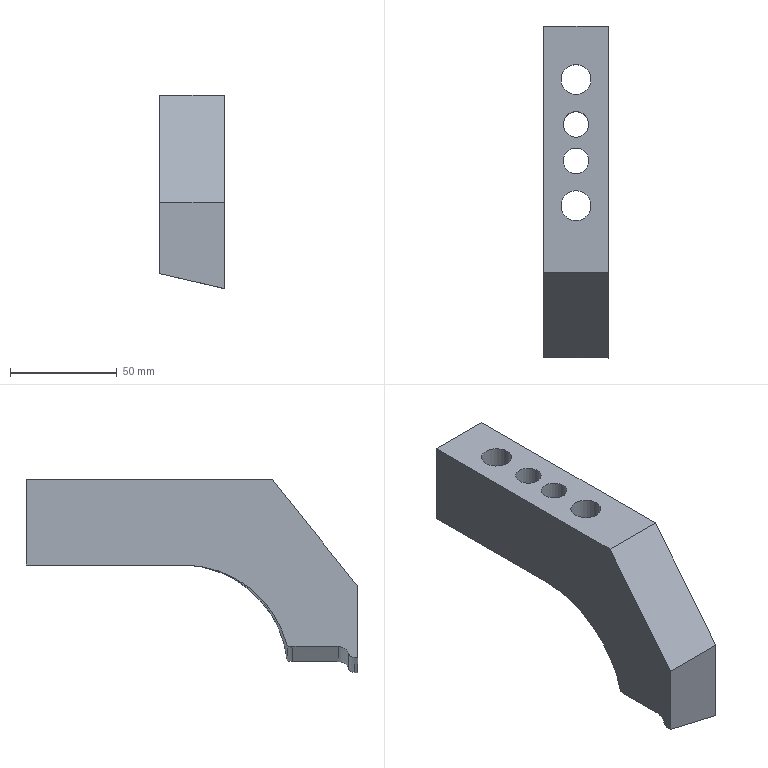Part | NX | features solid 2 | 1 solid | 21 faces | box 30 x 155 x 90.276 mm | volume 186324 mm3 | plane 8 | spline 7 | cylinder 6 | commonest cylinder face diameters 12 x2 14 x2 20 x2
STEP:
#1=CARTESIAN_POINT('',(-556.,-381.,60.));
#2=VERTEX_POINT('',#1);
#3=CARTESIAN_POINT('',(-550.,-381.,60.));
#4=DIRECTION('',(0.,0.,-1.));
#5=DIRECTION('',(-1.,0.,0.));
#6=AXIS2_PLACEMENT_3D('',#3,#4,#5);
#7=CIRCLE('',#6,6.);
#8=EDGE_CURVE('',#2,#2,#7,.T.);
#9=ORIENTED_EDGE('',*,*,#8,.F.);
#10=EDGE_LOOP('',(#9));
#11=FACE_BOUND('',#10,.T.);
#12=CARTESIAN_POINT('',(-556.,-364.,60.));
#13=VERTEX_POINT('',#12);
#14=CARTESIAN_POINT('',(-550.,-364.,60.));
#15=DIRECTION('',(0.,0.,-1.));
#16=DIRECTION('',(-1.,0.,0.));
#17=AXIS2_PLACEMENT_3D('',#14,#15,#16);
#18=CIRCLE('',#17,6.);
#19=EDGE_CURVE('',#13,#13,#18,.T.);
#20=ORIENTED_EDGE('',*,*,#19,.F.);
#21=EDGE_LOOP('',(#20));
#22=FACE_BOUND('',#21,.T.);
#23=CARTESIAN_POINT('',(-560.,-343.,60.));
#24=VERTEX_POINT('',#23);
#25=CARTESIAN_POINT('',(-550.,-343.,60.));
#26=DIRECTION('',(0.,0.,-1.));
#27=DIRECTION('',(-1.,0.,0.));
#28=AXIS2_PLACEMENT_3D('',#25,#26,#27);
#29=CIRCLE('',#28,10.);
#30=EDGE_CURVE('',#24,#24,#29,.F.);
#31=ORIENTED_EDGE('',*,*,#30,.T.);
#32=EDGE_LOOP('',(#31));
#33=FACE_BOUND('',#32,.T.);
#34=CARTESIAN_POINT('',(-535.,-390.262,60.));
#35=VERTEX_POINT('',#34);
#36=CARTESIAN_POINT('',(-535.,-318.,60.));
#37=VERTEX_POINT('',#36);
#38=CARTESIAN_POINT('',(-535.,-449.758,60.));
#39=DIRECTION('',(0.,1.,0.));
#40=VECTOR('',#39,1000.);
#41=LINE('',#38,#40);
#42=EDGE_CURVE('',#35,#37,#41,.T.);
#43=ORIENTED_EDGE('',*,*,#42,.F.);
#44=CARTESIAN_POINT('',(-565.,-391.431,60.));
#45=VERTEX_POINT('',#44);
#46=CARTESIAN_POINT('',(-535.,-390.262,60.));
#47=CARTESIAN_POINT('',(-545.006,-390.49,60.));
#48=CARTESIAN_POINT('',(-555.007,-390.87,60.));
#49=CARTESIAN_POINT('',(-565.,-391.431,60.));
#50=B_SPLINE_CURVE_WITH_KNOTS('',3,(#46,#47,#48,#49),.UNSPECIFIED.,.F.,.F.,(4,4),(0.,0.03002),.UNSPECIFIED.);
#51=EDGE_CURVE('',#35,#45,#50,.T.);
#52=ORIENTED_EDGE('',*,*,#51,.T.);
#53=CARTESIAN_POINT('',(-565.,-318.,60.));
#54=VERTEX_POINT('',#53);
#55=CARTESIAN_POINT('',(-565.,-425.,60.));
#56=DIRECTION('',(0.,1.,0.));
#57=VECTOR('',#56,1000.);
#58=LINE('',#55,#57);
#59=EDGE_CURVE('',#45,#54,#58,.T.);
#60=ORIENTED_EDGE('',*,*,#59,.T.);
#61=CARTESIAN_POINT('',(-535.,-318.,60.));
#62=CARTESIAN_POINT('',(-545.,-318.,60.));
#63=CARTESIAN_POINT('',(-555.,-318.,60.));
#64=CARTESIAN_POINT('',(-565.,-318.,60.));
#65=B_SPLINE_CURVE_WITH_KNOTS('',3,(#61,#62,#63,#64),.UNSPECIFIED.,.F.,.F.,(4,4),(0.,0.03),.UNSPECIFIED.);
#66=EDGE_CURVE('',#37,#54,#65,.T.);
#67=ORIENTED_EDGE('',*,*,#66,.F.);
#68=EDGE_LOOP('',(#43,#52,#60,#67));
#69=FACE_BOUND('',#68,.T.);
#70=CARTESIAN_POINT('',(-535.,-425.,60.));
#71=DIRECTION('',(0.,0.,-1.));
#72=DIRECTION('',(-1.,0.,0.));
#73=AXIS2_PLACEMENT_3D('',#70,#71,#72);
#74=PLANE('',#73);
#75=ADVANCED_FACE('',(#11,#22,#33,#69),#74,.T.);
#76=CARTESIAN_POINT('',(-565.,-473.,16.731));
#77=VERTEX_POINT('',#76);
#78=CARTESIAN_POINT('',(-565.,-473.,50.));
#79=VERTEX_POINT('',#78);
#80=CARTESIAN_POINT('',(-565.,-473.,75.));
#81=DIRECTION('',(0.,0.,-1.));
#82=VECTOR('',#81,1000.);
#83=LINE('',#80,#82);
#84=EDGE_CURVE('',#77,#79,#83,.F.);
#85=ORIENTED_EDGE('',*,*,#84,.T.);
#86=CARTESIAN_POINT('',(-565.,-433.,100.));
#87=VERTEX_POINT('',#86);
#88=CARTESIAN_POINT('',(-565.,-473.,50.));
#89=DIRECTION('',(0.,0.6247,0.7809));
#90=VECTOR('',#89,1000.);
#91=LINE('',#88,#90);
#92=EDGE_CURVE('',#79,#87,#91,.T.);
#93=ORIENTED_EDGE('',*,*,#92,.T.);
#94=CARTESIAN_POINT('',(-565.,-318.,100.));
#95=VERTEX_POINT('',#94);
#96=CARTESIAN_POINT('',(-565.,-425.,100.));
#97=DIRECTION('',(0.,-1.,0.));
#98=VECTOR('',#97,1000.);
#99=LINE('',#96,#98);
#100=EDGE_CURVE('',#87,#95,#99,.F.);
#101=ORIENTED_EDGE('',*,*,#100,.T.);
#102=CARTESIAN_POINT('',(-565.,-318.,60.));
#103=CARTESIAN_POINT('',(-565.,-318.,73.333));
#104=CARTESIAN_POINT('',(-565.,-318.,86.667));
#105=CARTESIAN_POINT('',(-565.,-318.,100.));
#106=B_SPLINE_CURVE_WITH_KNOTS('',3,(#102,#103,#104,#105),.UNSPECIFIED.,.F.,.F.,(4,4),(0.,0.04),.UNSPECIFIED.);
#107=EDGE_CURVE('',#54,#95,#106,.T.);
#108=ORIENTED_EDGE('',*,*,#107,.F.);
#109=ORIENTED_EDGE('',*,*,#59,.F.);
#110=CARTESIAN_POINT('',(-565.,-440.,22.203));
#111=VERTEX_POINT('',#110);
#112=CARTESIAN_POINT('',(-565.,-391.431,60.));
#113=CARTESIAN_POINT('',(-565.,-394.218,60.));
#114=CARTESIAN_POINT('',(-565.,-399.704,59.542));
#115=CARTESIAN_POINT('',(-565.,-407.765,57.509));
#116=CARTESIAN_POINT('',(-565.,-415.388,54.167));
#117=CARTESIAN_POINT('',(-565.,-422.329,49.641));
#118=CARTESIAN_POINT('',(-565.,-428.468,43.994));
#119=CARTESIAN_POINT('',(-565.,-433.553,37.471));
#120=CARTESIAN_POINT('',(-565.,-437.533,30.115));
#121=CARTESIAN_POINT('',(-565.,-439.319,24.906));
#122=CARTESIAN_POINT('',(-565.,-440.,22.203));
#123=B_SPLINE_CURVE_WITH_KNOTS('',3,(#112,#113,#114,#115,#116,#117,#118,#119,#120,#121,#122),.UNSPECIFIED.,.F.,.F.,(4,1,1,1,1,1,1,1,4),(0.,0.008243,0.01649,0.02473,0.03297,0.04121,0.04946,0.0577,0.06594),.UNSPECIFIED.);
#124=EDGE_CURVE('',#45,#111,#123,.T.);
#125=ORIENTED_EDGE('',*,*,#124,.T.);
#126=CARTESIAN_POINT('',(-565.,-442.207,21.944));
#127=VERTEX_POINT('',#126);
#128=CARTESIAN_POINT('',(-565.,-442.207,21.944));
#129=CARTESIAN_POINT('',(-565.,-441.46,21.946));
#130=CARTESIAN_POINT('',(-565.,-440.725,22.033));
#131=CARTESIAN_POINT('',(-565.,-440.,22.203));
#132=B_SPLINE_CURVE_WITH_KNOTS('',3,(#128,#129,#130,#131),.UNSPECIFIED.,.F.,.F.,(4,4),(0.000000091,0.002222),.UNSPECIFIED.);
#133=EDGE_CURVE('',#127,#111,#132,.T.);
#134=ORIENTED_EDGE('',*,*,#133,.F.);
#135=CARTESIAN_POINT('',(-565.,-464.022,21.891));
#136=VERTEX_POINT('',#135);
#137=CARTESIAN_POINT('',(-565.,-442.207,21.944));
#138=CARTESIAN_POINT('',(-565.,-449.479,21.926));
#139=CARTESIAN_POINT('',(-565.,-456.751,21.909));
#140=CARTESIAN_POINT('',(-565.,-464.022,21.891));
#141=B_SPLINE_CURVE_WITH_KNOTS('',3,(#137,#138,#139,#140),.UNSPECIFIED.,.F.,.F.,(4,4),(0.01263,0.03445),.UNSPECIFIED.);
#142=EDGE_CURVE('',#127,#136,#141,.T.);
#143=ORIENTED_EDGE('',*,*,#142,.T.);
#144=CARTESIAN_POINT('',(-565.,-468.65,18.668));
#145=VERTEX_POINT('',#144);
#146=CARTESIAN_POINT('',(-565.,-464.022,21.891));
#147=CARTESIAN_POINT('',(-565.,-466.037,21.887));
#148=CARTESIAN_POINT('',(-565.,-467.918,20.542));
#149=CARTESIAN_POINT('',(-565.,-468.65,18.668));
#150=B_SPLINE_CURVE_WITH_KNOTS('',3,(#146,#147,#148,#149),.UNSPECIFIED.,.F.,.F.,(4,4),(0.,0.005956),.UNSPECIFIED.);
#151=EDGE_CURVE('',#136,#145,#150,.T.);
#152=ORIENTED_EDGE('',*,*,#151,.T.);
#153=CARTESIAN_POINT('',(-565.,-471.431,16.734));
#154=VERTEX_POINT('',#153);
#155=CARTESIAN_POINT('',(-565.,-471.428,16.734));
#156=CARTESIAN_POINT('',(-565.,-470.829,16.737));
#157=CARTESIAN_POINT('',(-565.,-469.576,17.031));
#158=CARTESIAN_POINT('',(-565.,-468.869,18.107));
#159=CARTESIAN_POINT('',(-565.,-468.651,18.667));
#160=B_SPLINE_CURVE_WITH_KNOTS('',3,(#155,#156,#157,#158,#159),.UNSPECIFIED.,.F.,.F.,(4,1,4),(0.001586,0.003375,0.005164),.UNSPECIFIED.);
#161=EDGE_CURVE('',#154,#145,#160,.T.);
#162=ORIENTED_EDGE('',*,*,#161,.F.);
#163=CARTESIAN_POINT('',(-565.,-471.437,16.734));
#164=CARTESIAN_POINT('',(-565.,-471.958,16.733));
#165=CARTESIAN_POINT('',(-565.,-472.479,16.732));
#166=CARTESIAN_POINT('',(-565.,-473.,16.731));
#167=B_SPLINE_CURVE_WITH_KNOTS('',3,(#163,#164,#165,#166),.UNSPECIFIED.,.F.,.F.,(4,4),(0.005792,0.007355),.UNSPECIFIED.);
#168=EDGE_CURVE('',#154,#77,#167,.T.);
#169=ORIENTED_EDGE('',*,*,#168,.T.);
#170=EDGE_LOOP('',(#85,#93,#101,#108,#109,#125,#134,#143,#152,#162,#169));
#171=FACE_BOUND('',#170,.T.);
#172=CARTESIAN_POINT('',(-565.,-425.,75.));
#173=DIRECTION('',(1.,0.,0.));
#174=DIRECTION('',(0.,0.,-1.));
#175=AXIS2_PLACEMENT_3D('',#172,#173,#174);
#176=PLANE('',#175);
#177=ADVANCED_FACE('',(#171),#176,.F.);
#178=CARTESIAN_POINT('',(-535.,-433.,100.));
#179=VERTEX_POINT('',#178);
#180=CARTESIAN_POINT('',(-535.,-318.,100.));
#181=VERTEX_POINT('',#180);
#182=CARTESIAN_POINT('',(-535.,-425.,100.));
#183=DIRECTION('',(0.,-1.,0.));
#184=VECTOR('',#183,1000.);
#185=LINE('',#182,#184);
#186=EDGE_CURVE('',#179,#181,#185,.F.);
#187=ORIENTED_EDGE('',*,*,#186,.F.);
#188=CARTESIAN_POINT('',(-535.,-473.,50.));
#189=VERTEX_POINT('',#188);
#190=CARTESIAN_POINT('',(-535.,-585.881,-91.102));
#191=DIRECTION('',(0.,-0.6247,-0.7809));
#192=VECTOR('',#191,1000.);
#193=LINE('',#190,#192);
#194=EDGE_CURVE('',#179,#189,#193,.T.);
#195=ORIENTED_EDGE('',*,*,#194,.T.);
#196=CARTESIAN_POINT('',(-535.,-473.,9.724));
#197=VERTEX_POINT('',#196);
#198=CARTESIAN_POINT('',(-535.,-473.,-200.));
#199=DIRECTION('',(0.,0.,-1.));
#200=VECTOR('',#199,1000.);
#201=LINE('',#198,#200);
#202=EDGE_CURVE('',#197,#189,#201,.F.);
#203=ORIENTED_EDGE('',*,*,#202,.F.);
#204=CARTESIAN_POINT('',(-535.,-471.431,9.728));
#205=VERTEX_POINT('',#204);
#206=CARTESIAN_POINT('',(-535.,-471.438,9.728));
#207=CARTESIAN_POINT('',(-535.,-471.959,9.726));
#208=CARTESIAN_POINT('',(-535.,-472.479,9.725));
#209=CARTESIAN_POINT('',(-535.,-473.,9.724));
#210=B_SPLINE_CURVE_WITH_KNOTS('',3,(#206,#207,#208,#209),.UNSPECIFIED.,.F.,.F.,(4,4),(0.005813,0.007375),.UNSPECIFIED.);
#211=EDGE_CURVE('',#205,#197,#210,.T.);
#212=ORIENTED_EDGE('',*,*,#211,.F.);
#213=CARTESIAN_POINT('',(-535.,-468.651,11.657));
#214=VERTEX_POINT('',#213);
#215=CARTESIAN_POINT('',(-535.,-471.428,9.728));
#216=CARTESIAN_POINT('',(-535.,-470.823,9.731));
#217=CARTESIAN_POINT('',(-535.,-469.58,10.023));
#218=CARTESIAN_POINT('',(-535.,-468.869,11.097));
#219=CARTESIAN_POINT('',(-535.,-468.651,11.656));
#220=B_SPLINE_CURVE_WITH_KNOTS('',3,(#215,#216,#217,#218,#219),.UNSPECIFIED.,.F.,.F.,(4,1,4),(0.001587,0.003388,0.005189),.UNSPECIFIED.);
#221=EDGE_CURVE('',#205,#214,#220,.T.);
#222=ORIENTED_EDGE('',*,*,#221,.T.);
#223=CARTESIAN_POINT('',(-535.,-464.022,14.875));
#224=VERTEX_POINT('',#223);
#225=CARTESIAN_POINT('',(-535.,-464.022,14.875));
#226=CARTESIAN_POINT('',(-535.,-466.035,14.87));
#227=CARTESIAN_POINT('',(-535.,-467.917,13.53));
#228=CARTESIAN_POINT('',(-535.,-468.65,11.658));
#229=B_SPLINE_CURVE_WITH_KNOTS('',3,(#225,#226,#227,#228),.UNSPECIFIED.,.F.,.F.,(4,4),(0.,0.005952),.UNSPECIFIED.);
#230=EDGE_CURVE('',#224,#214,#229,.T.);
#231=ORIENTED_EDGE('',*,*,#230,.F.);
#232=CARTESIAN_POINT('',(-535.,-442.454,14.927));
#233=VERTEX_POINT('',#232);
#234=CARTESIAN_POINT('',(-535.,-442.454,14.927));
#235=CARTESIAN_POINT('',(-535.,-449.644,14.909));
#236=CARTESIAN_POINT('',(-535.,-456.833,14.891));
#237=CARTESIAN_POINT('',(-535.,-464.022,14.875));
#238=B_SPLINE_CURVE_WITH_KNOTS('',3,(#234,#235,#236,#237),.UNSPECIFIED.,.F.,.F.,(4,4),(0.0129,0.03447),.UNSPECIFIED.);
#239=EDGE_CURVE('',#233,#224,#238,.T.);
#240=ORIENTED_EDGE('',*,*,#239,.F.);
#241=CARTESIAN_POINT('',(-535.,-440.,15.246));
#242=VERTEX_POINT('',#241);
#243=CARTESIAN_POINT('',(-535.,-442.454,14.927));
#244=CARTESIAN_POINT('',(-535.,-441.622,14.929));
#245=CARTESIAN_POINT('',(-535.,-440.804,15.036));
#246=CARTESIAN_POINT('',(-535.,-440.,15.246));
#247=B_SPLINE_CURVE_WITH_KNOTS('',3,(#243,#244,#245,#246),.UNSPECIFIED.,.F.,.F.,(4,4),(0.,0.002475),.UNSPECIFIED.);
#248=EDGE_CURVE('',#233,#242,#247,.T.);
#249=ORIENTED_EDGE('',*,*,#248,.T.);
#250=CARTESIAN_POINT('',(-535.,-440.,15.246));
#251=CARTESIAN_POINT('',(-535.,-439.677,18.311));
#252=CARTESIAN_POINT('',(-535.,-438.488,24.267));
#253=CARTESIAN_POINT('',(-535.,-435.058,32.858));
#254=CARTESIAN_POINT('',(-535.,-430.185,40.582));
#255=CARTESIAN_POINT('',(-535.,-423.893,47.384));
#256=CARTESIAN_POINT('',(-535.,-416.594,52.839));
#257=CARTESIAN_POINT('',(-535.,-408.272,56.946));
#258=CARTESIAN_POINT('',(-535.,-399.512,59.42));
#259=CARTESIAN_POINT('',(-535.,-393.344,60.));
#260=CARTESIAN_POINT('',(-535.,-390.262,60.));
#261=B_SPLINE_CURVE_WITH_KNOTS('',3,(#250,#251,#252,#253,#254,#255,#256,#257,#258,#259,#260),.UNSPECIFIED.,.F.,.F.,(4,1,1,1,1,1,1,1,4),(0.,0.009112,0.01822,0.02734,0.03645,0.04556,0.05467,0.06379,0.0729),.UNSPECIFIED.);
#262=EDGE_CURVE('',#242,#35,#261,.T.);
#263=ORIENTED_EDGE('',*,*,#262,.T.);
#264=ORIENTED_EDGE('',*,*,#42,.T.);
#265=CARTESIAN_POINT('',(-535.,-318.,60.));
#266=CARTESIAN_POINT('',(-535.,-318.,73.333));
#267=CARTESIAN_POINT('',(-535.,-318.,86.667));
#268=CARTESIAN_POINT('',(-535.,-318.,100.));
#269=B_SPLINE_CURVE_WITH_KNOTS('',3,(#265,#266,#267,#268),.UNSPECIFIED.,.F.,.F.,(4,4),(0.,0.04),.UNSPECIFIED.);
#270=EDGE_CURVE('',#37,#181,#269,.T.);
#271=ORIENTED_EDGE('',*,*,#270,.T.);
#272=EDGE_LOOP('',(#187,#195,#203,#212,#222,#231,#240,#249,#263,#264,#271));
#273=FACE_BOUND('',#272,.T.);
#274=CARTESIAN_POINT('',(-535.,-449.758,-200.));
#275=DIRECTION('',(1.,0.,0.));
#276=DIRECTION('',(0.,0.,-1.));
#277=AXIS2_PLACEMENT_3D('',#274,#275,#276);
#278=PLANE('',#277);
#279=ADVANCED_FACE('',(#273),#278,.T.);
#280=ORIENTED_EDGE('',*,*,#202,.T.);
#281=CARTESIAN_POINT('',(-565.,-473.,50.));
#282=DIRECTION('',(1.,0.,0.));
#283=VECTOR('',#282,1000.);
#284=LINE('',#281,#283);
#285=EDGE_CURVE('',#189,#79,#284,.F.);
#286=ORIENTED_EDGE('',*,*,#285,.T.);
#287=ORIENTED_EDGE('',*,*,#84,.F.);
#288=CARTESIAN_POINT('',(-565.,-473.,16.731));
#289=CARTESIAN_POINT('',(-555.01,-473.,14.353));
#290=CARTESIAN_POINT('',(-545.01,-473.,12.017));
#291=CARTESIAN_POINT('',(-535.,-473.,9.724));
#292=B_SPLINE_CURVE_WITH_KNOTS('',3,(#288,#289,#290,#291),.UNSPECIFIED.,.F.,.F.,(4,4),(0.,0.03081),.UNSPECIFIED.);
#293=EDGE_CURVE('',#77,#197,#292,.T.);
#294=ORIENTED_EDGE('',*,*,#293,.T.);
#295=EDGE_LOOP('',(#280,#286,#287,#294));
#296=FACE_BOUND('',#295,.T.);
#297=CARTESIAN_POINT('',(-535.,-473.,60.));
#298=DIRECTION('',(0.,-1.,0.));
#299=DIRECTION('',(-1.,0.,0.));
#300=AXIS2_PLACEMENT_3D('',#297,#298,#299);
#301=PLANE('',#300);
#302=ADVANCED_FACE('',(#296),#301,.T.);
#303=ORIENTED_EDGE('',*,*,#270,.F.);
#304=ORIENTED_EDGE('',*,*,#66,.T.);
#305=ORIENTED_EDGE('',*,*,#107,.T.);
#306=CARTESIAN_POINT('',(-535.,-318.,100.));
#307=CARTESIAN_POINT('',(-545.,-318.,100.));
#308=CARTESIAN_POINT('',(-555.,-318.,100.));
#309=CARTESIAN_POINT('',(-565.,-318.,100.));
#310=B_SPLINE_CURVE_WITH_KNOTS('',3,(#306,#307,#308,#309),.UNSPECIFIED.,.F.,.F.,(4,4),(0.,0.03),.UNSPECIFIED.);
#311=EDGE_CURVE('',#181,#95,#310,.T.);
#312=ORIENTED_EDGE('',*,*,#311,.F.);
#313=EDGE_LOOP('',(#303,#304,#305,#312));
#314=FACE_BOUND('',#313,.T.);
#315=CARTESIAN_POINT('',(-565.,-318.,100.));
#316=CARTESIAN_POINT('',(-535.,-318.,100.));
#317=CARTESIAN_POINT('',(-565.,-318.,60.));
#318=CARTESIAN_POINT('',(-535.,-318.,60.));
#319=B_SPLINE_SURFACE_WITH_KNOTS('',1,1,((#315,#316),(#317,#318)),.PLANE_SURF.,.F.,.F.,.F.,(2,2),(2,2),(0.3333,0.4137),(-3.556,-3.222),.PIECEWISE_BEZIER_KNOTS.);
#320=ADVANCED_FACE('',(#314),#319,.F.);
#321=CARTESIAN_POINT('',(-540.,-343.,75.));
#322=VERTEX_POINT('',#321);
#323=CARTESIAN_POINT('',(-550.,-343.,75.));
#324=DIRECTION('',(0.,0.,-1.));
#325=DIRECTION('',(1.,0.,0.));
#326=AXIS2_PLACEMENT_3D('',#323,#324,#325);
#327=CIRCLE('',#326,10.);
#328=EDGE_CURVE('',#322,#322,#327,.T.);
#329=ORIENTED_EDGE('',*,*,#328,.F.);
#330=EDGE_LOOP('',(#329));
#331=FACE_BOUND('',#330,.T.);
#332=ORIENTED_EDGE('',*,*,#30,.F.);
#333=EDGE_LOOP('',(#332));
#334=FACE_BOUND('',#333,.T.);
#335=CARTESIAN_POINT('',(-550.,-343.,75.));
#336=DIRECTION('',(0.,0.,-1.));
#337=DIRECTION('',(1.,0.,0.));
#338=AXIS2_PLACEMENT_3D('',#335,#336,#337);
#339=CYLINDRICAL_SURFACE('',#338,10.);
#340=ADVANCED_FACE('',(#331,#334),#339,.F.);
#341=CARTESIAN_POINT('',(-540.,-402.,75.));
#342=VERTEX_POINT('',#341);
#343=CARTESIAN_POINT('',(-550.,-402.,75.));
#344=DIRECTION('',(0.,0.,-1.));
#345=DIRECTION('',(1.,0.,0.));
#346=AXIS2_PLACEMENT_3D('',#343,#344,#345);
#347=CIRCLE('',#346,10.);
#348=EDGE_CURVE('',#342,#342,#347,.T.);
#349=ORIENTED_EDGE('',*,*,#348,.F.);
#350=EDGE_LOOP('',(#349));
#351=FACE_BOUND('',#350,.T.);
#352=CARTESIAN_POINT('',(-540.005,-401.699,58.705));
#353=VERTEX_POINT('',#352);
#354=CARTESIAN_POINT('',(-541.365,-408.115,56.844));
#355=CARTESIAN_POINT('',(-539.449,-403.012,58.517));
#356=CARTESIAN_POINT('',(-540.637,-397.798,59.499));
#357=CARTESIAN_POINT('',(-543.77,-393.388,59.985));
#358=CARTESIAN_POINT('',(-550.513,-390.886,59.985));
#359=CARTESIAN_POINT('',(-557.01,-394.007,59.981));
#360=CARTESIAN_POINT('',(-559.716,-398.695,59.478));
#361=CARTESIAN_POINT('',(-560.409,-403.985,58.477));
#362=CARTESIAN_POINT('',(-558.038,-408.878,56.801));
#363=CARTESIAN_POINT('',(-553.557,-411.624,55.503));
#364=CARTESIAN_POINT('',(-549.536,-412.263,55.118));
#365=CARTESIAN_POINT('',(-545.585,-411.262,55.527));
#366=CARTESIAN_POINT('',(-541.365,-408.115,56.844));
#367=CARTESIAN_POINT('',(-539.449,-403.012,58.517));
#368=CARTESIAN_POINT('',(-540.637,-397.798,59.499));
#369=B_SPLINE_CURVE_WITH_KNOTS('',3,(#354,#355,#356,#357,#358,#359,#360,#361,#362,#363,#364,#365,#366,#367,#368),.UNSPECIFIED.,.T.,.F.,(1,1,1,1,1,1,1,1,1,1,1,1,1,1,1,1,1,1,1),(-0.01589,-0.01192,-0.007945,0.,0.003973,0.007945,0.01589,0.02384,0.02781,0.03178,0.03973,0.0437,0.04767,0.05165,0.05562,0.06356,0.06754,0.07151,0.07945),.UNSPECIFIED.);
#370=EDGE_CURVE('',#353,#353,#369,.T.);
#371=ORIENTED_EDGE('',*,*,#370,.F.);
#372=EDGE_LOOP('',(#371));
#373=FACE_BOUND('',#372,.T.);
#374=CARTESIAN_POINT('',(-550.,-402.,75.));
#375=DIRECTION('',(0.,0.,-1.));
#376=DIRECTION('',(1.,0.,0.));
#377=AXIS2_PLACEMENT_3D('',#374,#375,#376);
#378=CYLINDRICAL_SURFACE('',#377,10.);
#379=ADVANCED_FACE('',(#351,#373),#378,.F.);
#380=ORIENTED_EDGE('',*,*,#100,.F.);
#381=CARTESIAN_POINT('',(-535.,-433.,100.));
#382=DIRECTION('',(-1.,0.,0.));
#383=VECTOR('',#382,1000.);
#384=LINE('',#381,#383);
#385=EDGE_CURVE('',#87,#179,#384,.F.);
#386=ORIENTED_EDGE('',*,*,#385,.T.);
#387=ORIENTED_EDGE('',*,*,#186,.T.);
#388=ORIENTED_EDGE('',*,*,#311,.T.);
#389=EDGE_LOOP('',(#380,#386,#387,#388));
#390=FACE_BOUND('',#389,.T.);
#391=CARTESIAN_POINT('',(-556.,-381.,100.));
#392=VERTEX_POINT('',#391);
#393=CARTESIAN_POINT('',(-550.,-381.,100.));
#394=DIRECTION('',(0.,0.,-1.));
#395=DIRECTION('',(-1.,0.,0.));
#396=AXIS2_PLACEMENT_3D('',#393,#394,#395);
#397=CIRCLE('',#396,6.);
#398=EDGE_CURVE('',#392,#392,#397,.T.);
#399=ORIENTED_EDGE('',*,*,#398,.T.);
#400=EDGE_LOOP('',(#399));
#401=FACE_BOUND('',#400,.T.);
#402=CARTESIAN_POINT('',(-556.,-364.,100.));
#403=VERTEX_POINT('',#402);
#404=CARTESIAN_POINT('',(-550.,-364.,100.));
#405=DIRECTION('',(0.,0.,-1.));
#406=DIRECTION('',(-1.,0.,0.));
#407=AXIS2_PLACEMENT_3D('',#404,#405,#406);
#408=CIRCLE('',#407,6.);
#409=EDGE_CURVE('',#403,#403,#408,.T.);
#410=ORIENTED_EDGE('',*,*,#409,.T.);
#411=EDGE_LOOP('',(#410));
#412=FACE_BOUND('',#411,.T.);
#413=CARTESIAN_POINT('',(-557.,-402.,100.));
#414=VERTEX_POINT('',#413);
#415=CARTESIAN_POINT('',(-550.,-402.,100.));
#416=DIRECTION('',(0.,0.,-1.));
#417=DIRECTION('',(-1.,0.,0.));
#418=AXIS2_PLACEMENT_3D('',#415,#416,#417);
#419=CIRCLE('',#418,7.);
#420=EDGE_CURVE('',#414,#414,#419,.T.);
#421=ORIENTED_EDGE('',*,*,#420,.T.);
#422=EDGE_LOOP('',(#421));
#423=FACE_BOUND('',#422,.T.);
#424=CARTESIAN_POINT('',(-557.,-343.,100.));
#425=VERTEX_POINT('',#424);
#426=CARTESIAN_POINT('',(-550.,-343.,100.));
#427=DIRECTION('',(0.,0.,-1.));
#428=DIRECTION('',(-1.,0.,0.));
#429=AXIS2_PLACEMENT_3D('',#426,#427,#428);
#430=CIRCLE('',#429,7.);
#431=EDGE_CURVE('',#425,#425,#430,.T.);
#432=ORIENTED_EDGE('',*,*,#431,.T.);
#433=EDGE_LOOP('',(#432));
#434=FACE_BOUND('',#433,.T.);
#435=CARTESIAN_POINT('',(-605.,-425.,100.));
#436=DIRECTION('',(0.,0.,-1.));
#437=DIRECTION('',(-1.,0.,0.));
#438=AXIS2_PLACEMENT_3D('',#435,#436,#437);
#439=PLANE('',#438);
#440=ADVANCED_FACE('',(#390,#401,#412,#423,#434),#439,.F.);
#441=CARTESIAN_POINT('',(-543.,-343.,75.));
#442=VERTEX_POINT('',#441);
#443=CARTESIAN_POINT('',(-550.,-343.,75.));
#444=DIRECTION('',(0.,0.,1.));
#445=DIRECTION('',(1.,0.,0.));
#446=AXIS2_PLACEMENT_3D('',#443,#444,#445);
#447=CIRCLE('',#446,7.);
#448=EDGE_CURVE('',#442,#442,#447,.T.);
#449=ORIENTED_EDGE('',*,*,#448,.F.);
#450=EDGE_LOOP('',(#449));
#451=FACE_BOUND('',#450,.T.);
#452=ORIENTED_EDGE('',*,*,#431,.F.);
#453=EDGE_LOOP('',(#452));
#454=FACE_BOUND('',#453,.T.);
#455=CARTESIAN_POINT('',(-550.,-343.,75.));
#456=DIRECTION('',(0.,0.,1.));
#457=DIRECTION('',(-1.,0.,0.));
#458=AXIS2_PLACEMENT_3D('',#455,#456,#457);
#459=CYLINDRICAL_SURFACE('',#458,7.);
#460=ADVANCED_FACE('',(#451,#454),#459,.F.);
#461=ORIENTED_EDGE('',*,*,#448,.T.);
#462=EDGE_LOOP('',(#461));
#463=FACE_BOUND('',#462,.T.);
#464=ORIENTED_EDGE('',*,*,#328,.T.);
#465=EDGE_LOOP('',(#464));
#466=FACE_BOUND('',#465,.T.);
#467=CARTESIAN_POINT('',(-550.,-343.,75.));
#468=DIRECTION('',(0.,0.,1.));
#469=DIRECTION('',(-1.,0.,0.));
#470=AXIS2_PLACEMENT_3D('',#467,#468,#469);
#471=PLANE('',#470);
#472=ADVANCED_FACE('',(#463,#466),#471,.F.);
#473=CARTESIAN_POINT('',(-543.,-402.,75.));
#474=VERTEX_POINT('',#473);
#475=CARTESIAN_POINT('',(-550.,-402.,75.));
#476=DIRECTION('',(0.,0.,1.));
#477=DIRECTION('',(1.,0.,0.));
#478=AXIS2_PLACEMENT_3D('',#475,#476,#477);
#479=CIRCLE('',#478,7.);
#480=EDGE_CURVE('',#474,#474,#479,.T.);
#481=ORIENTED_EDGE('',*,*,#480,.F.);
#482=EDGE_LOOP('',(#481));
#483=FACE_BOUND('',#482,.T.);
#484=ORIENTED_EDGE('',*,*,#420,.F.);
#485=EDGE_LOOP('',(#484));
#486=FACE_BOUND('',#485,.T.);
#487=CARTESIAN_POINT('',(-550.,-402.,75.));
#488=DIRECTION('',(0.,0.,1.));
#489=DIRECTION('',(-1.,0.,0.));
#490=AXIS2_PLACEMENT_3D('',#487,#488,#489);
#491=CYLINDRICAL_SURFACE('',#490,7.);
#492=ADVANCED_FACE('',(#483,#486),#491,.F.);
#493=ORIENTED_EDGE('',*,*,#480,.T.);
#494=EDGE_LOOP('',(#493));
#495=FACE_BOUND('',#494,.T.);
#496=ORIENTED_EDGE('',*,*,#348,.T.);
#497=EDGE_LOOP('',(#496));
#498=FACE_BOUND('',#497,.T.);
#499=CARTESIAN_POINT('',(-550.,-402.,75.));
#500=DIRECTION('',(0.,0.,1.));
#501=DIRECTION('',(-1.,0.,0.));
#502=AXIS2_PLACEMENT_3D('',#499,#500,#501);
#503=PLANE('',#502);
#504=ADVANCED_FACE('',(#495,#498),#503,.F.);
#505=ORIENTED_EDGE('',*,*,#409,.F.);
#506=EDGE_LOOP('',(#505));
#507=FACE_BOUND('',#506,.T.);
#508=ORIENTED_EDGE('',*,*,#19,.T.);
#509=EDGE_LOOP('',(#508));
#510=FACE_BOUND('',#509,.T.);
#511=CARTESIAN_POINT('',(-550.,-364.,105.));
#512=DIRECTION('',(0.,0.,-1.));
#513=DIRECTION('',(-1.,0.,0.));
#514=AXIS2_PLACEMENT_3D('',#511,#512,#513);
#515=CYLINDRICAL_SURFACE('',#514,6.);
#516=ADVANCED_FACE('',(#507,#510),#515,.F.);
#517=ORIENTED_EDGE('',*,*,#398,.F.);
#518=EDGE_LOOP('',(#517));
#519=FACE_BOUND('',#518,.T.);
#520=ORIENTED_EDGE('',*,*,#8,.T.);
#521=EDGE_LOOP('',(#520));
#522=FACE_BOUND('',#521,.T.);
#523=CARTESIAN_POINT('',(-550.,-381.,105.));
#524=DIRECTION('',(0.,0.,-1.));
#525=DIRECTION('',(-1.,0.,0.));
#526=AXIS2_PLACEMENT_3D('',#523,#524,#525);
#527=CYLINDRICAL_SURFACE('',#526,6.);
#528=ADVANCED_FACE('',(#519,#522),#527,.F.);
#529=ORIENTED_EDGE('',*,*,#161,.T.);
#530=CARTESIAN_POINT('',(-565.,-468.651,18.667));
#531=CARTESIAN_POINT('',(-554.961,-468.651,16.276));
#532=CARTESIAN_POINT('',(-544.961,-468.651,13.939));
#533=CARTESIAN_POINT('',(-535.,-468.651,11.656));
#534=B_SPLINE_CURVE_WITH_KNOTS('',3,(#530,#531,#532,#533),.UNSPECIFIED.,.F.,.F.,(4,4),(0.1684,0.2187),.UNSPECIFIED.);
#535=EDGE_CURVE('',#145,#214,#534,.T.);
#536=ORIENTED_EDGE('',*,*,#535,.T.);
#537=ORIENTED_EDGE('',*,*,#221,.F.);
#538=CARTESIAN_POINT('',(-535.,-471.428,9.728));
#539=CARTESIAN_POINT('',(-544.961,-471.428,12.009));
#540=CARTESIAN_POINT('',(-554.961,-471.428,14.345));
#541=CARTESIAN_POINT('',(-565.,-471.428,16.734));
#542=B_SPLINE_CURVE_WITH_KNOTS('',3,(#538,#539,#540,#541),.UNSPECIFIED.,.F.,.F.,(4,4),(0.7815,0.8318),.UNSPECIFIED.);
#543=EDGE_CURVE('',#205,#154,#542,.T.);
#544=ORIENTED_EDGE('',*,*,#543,.T.);
#545=EDGE_LOOP('',(#529,#536,#537,#544));
#546=FACE_BOUND('',#545,.T.);
#547=CARTESIAN_POINT('',(-534.818,-471.454,9.686));
#548=CARTESIAN_POINT('',(-534.815,-470.946,9.685));
#549=CARTESIAN_POINT('',(-534.802,-470.489,9.755));
#550=CARTESIAN_POINT('',(-534.777,-470.083,9.895));
#551=CARTESIAN_POINT('',(-534.706,-469.383,10.311));
#552=CARTESIAN_POINT('',(-534.593,-468.875,10.994));
#553=CARTESIAN_POINT('',(-534.527,-468.67,11.394));
#554=CARTESIAN_POINT('',(-534.435,-468.475,11.96));
#555=CARTESIAN_POINT('',(-534.327,-468.349,12.621));
#556=CARTESIAN_POINT('',(-534.307,-468.328,12.745));
#557=CARTESIAN_POINT('',(-534.287,-468.31,12.872));
#558=CARTESIAN_POINT('',(-534.266,-468.293,13.002));
#559=CARTESIAN_POINT('',(-535.373,-471.477,9.813));
#560=CARTESIAN_POINT('',(-535.371,-470.967,9.809));
#561=CARTESIAN_POINT('',(-535.358,-470.509,9.877));
#562=CARTESIAN_POINT('',(-535.333,-470.101,10.015));
#563=CARTESIAN_POINT('',(-535.263,-469.397,10.425));
#564=CARTESIAN_POINT('',(-535.151,-468.885,11.103));
#565=CARTESIAN_POINT('',(-535.085,-468.679,11.501));
#566=CARTESIAN_POINT('',(-534.994,-468.482,12.064));
#567=CARTESIAN_POINT('',(-534.887,-468.354,12.722));
#568=CARTESIAN_POINT('',(-534.867,-468.332,12.846));
#569=CARTESIAN_POINT('',(-534.846,-468.313,12.972));
#570=CARTESIAN_POINT('',(-534.825,-468.297,13.102));
#571=CARTESIAN_POINT('',(-535.928,-471.5,9.941));
#572=CARTESIAN_POINT('',(-535.926,-470.989,9.934));
#573=CARTESIAN_POINT('',(-535.913,-470.528,9.999));
#574=CARTESIAN_POINT('',(-535.889,-470.119,10.134));
#575=CARTESIAN_POINT('',(-535.82,-469.411,10.54));
#576=CARTESIAN_POINT('',(-535.709,-468.896,11.213));
#577=CARTESIAN_POINT('',(-535.644,-468.688,11.608));
#578=CARTESIAN_POINT('',(-535.552,-468.489,12.168));
#579=CARTESIAN_POINT('',(-535.446,-468.358,12.824));
#580=CARTESIAN_POINT('',(-535.426,-468.337,12.947));
#581=CARTESIAN_POINT('',(-535.406,-468.317,13.072));
#582=CARTESIAN_POINT('',(-535.385,-468.3,13.201));
#583=CARTESIAN_POINT('',(-536.483,-471.524,10.068));
#584=CARTESIAN_POINT('',(-536.482,-471.01,10.059));
#585=CARTESIAN_POINT('',(-536.469,-470.548,10.121));
#586=CARTESIAN_POINT('',(-536.446,-470.137,10.254));
#587=CARTESIAN_POINT('',(-536.377,-469.426,10.655));
#588=CARTESIAN_POINT('',(-536.266,-468.907,11.323));
#589=CARTESIAN_POINT('',(-536.202,-468.697,11.715));
#590=CARTESIAN_POINT('',(-536.111,-468.496,12.273));
#591=CARTESIAN_POINT('',(-536.005,-468.363,12.925));
#592=CARTESIAN_POINT('',(-535.985,-468.341,13.048));
#593=CARTESIAN_POINT('',(-535.965,-468.321,13.173));
#594=CARTESIAN_POINT('',(-535.944,-468.304,13.301));
#595=CARTESIAN_POINT('',(-542.624,-471.787,11.484));
#596=CARTESIAN_POINT('',(-542.627,-471.253,11.445));
#597=CARTESIAN_POINT('',(-542.619,-470.77,11.479));
#598=CARTESIAN_POINT('',(-542.599,-470.338,11.583));
#599=CARTESIAN_POINT('',(-542.54,-469.586,11.927));
#600=CARTESIAN_POINT('',(-542.438,-469.028,12.54));
#601=CARTESIAN_POINT('',(-542.377,-468.798,12.906));
#602=CARTESIAN_POINT('',(-542.292,-468.574,13.431));
#603=CARTESIAN_POINT('',(-542.191,-468.418,14.05));
#604=CARTESIAN_POINT('',(-542.172,-468.392,14.167));
#605=CARTESIAN_POINT('',(-542.153,-468.368,14.286));
#606=CARTESIAN_POINT('',(-542.133,-468.346,14.409));
#607=CARTESIAN_POINT('',(-548.759,-472.074,12.932));
#608=CARTESIAN_POINT('',(-548.766,-471.518,12.863));
#609=CARTESIAN_POINT('',(-548.763,-471.013,12.866));
#610=CARTESIAN_POINT('',(-548.749,-470.559,12.94));
#611=CARTESIAN_POINT('',(-548.698,-469.765,13.225));
#612=CARTESIAN_POINT('',(-548.605,-469.166,13.781));
#613=CARTESIAN_POINT('',(-548.549,-468.917,14.119));
#614=CARTESIAN_POINT('',(-548.469,-468.668,14.61));
#615=CARTESIAN_POINT('',(-548.373,-468.487,15.196));
#616=CARTESIAN_POINT('',(-548.355,-468.457,15.306));
#617=CARTESIAN_POINT('',(-548.337,-468.428,15.419));
#618=CARTESIAN_POINT('',(-548.318,-468.402,15.536));
#619=CARTESIAN_POINT('',(-554.334,-472.356,14.278));
#620=CARTESIAN_POINT('',(-554.347,-471.779,14.181));
#621=CARTESIAN_POINT('',(-554.348,-471.254,14.156));
#622=CARTESIAN_POINT('',(-554.338,-470.78,14.201));
#623=CARTESIAN_POINT('',(-554.296,-469.946,14.431));
#624=CARTESIAN_POINT('',(-554.212,-469.308,14.933));
#625=CARTESIAN_POINT('',(-554.16,-469.04,15.245));
#626=CARTESIAN_POINT('',(-554.084,-468.768,15.704));
#627=CARTESIAN_POINT('',(-553.994,-468.565,16.258));
#628=CARTESIAN_POINT('',(-553.977,-468.53,16.362));
#629=CARTESIAN_POINT('',(-553.96,-468.497,16.469));
#630=CARTESIAN_POINT('',(-553.942,-468.467,16.58));
#631=CARTESIAN_POINT('',(-559.905,-472.661,15.657));
#632=CARTESIAN_POINT('',(-559.922,-472.063,15.53));
#633=CARTESIAN_POINT('',(-559.928,-471.516,15.475));
#634=CARTESIAN_POINT('',(-559.923,-471.021,15.491));
#635=CARTESIAN_POINT('',(-559.89,-470.146,15.663));
#636=CARTESIAN_POINT('',(-559.815,-469.467,16.109));
#637=CARTESIAN_POINT('',(-559.767,-469.18,16.393));
#638=CARTESIAN_POINT('',(-559.697,-468.884,16.819));
#639=CARTESIAN_POINT('',(-559.611,-468.657,17.34));
#640=CARTESIAN_POINT('',(-559.595,-468.618,17.439));
#641=CARTESIAN_POINT('',(-559.579,-468.581,17.54));
#642=CARTESIAN_POINT('',(-559.562,-468.546,17.644));
#643=CARTESIAN_POINT('',(-565.471,-472.99,17.068));
#644=CARTESIAN_POINT('',(-565.493,-472.37,16.911));
#645=CARTESIAN_POINT('',(-565.503,-471.802,16.826));
#646=CARTESIAN_POINT('',(-565.503,-471.285,16.812));
#647=CARTESIAN_POINT('',(-565.479,-470.367,16.925));
#648=CARTESIAN_POINT('',(-565.413,-469.646,17.311));
#649=CARTESIAN_POINT('',(-565.37,-469.338,17.568));
#650=CARTESIAN_POINT('',(-565.305,-469.018,17.959));
#651=CARTESIAN_POINT('',(-565.225,-468.766,18.446));
#652=CARTESIAN_POINT('',(-565.21,-468.722,18.538));
#653=CARTESIAN_POINT('',(-565.194,-468.681,18.634));
#654=CARTESIAN_POINT('',(-565.178,-468.642,18.732));
#655=B_SPLINE_SURFACE_WITH_KNOTS('',5,5,((#547,#548,#549,#550,#551,#552,#553,#554,#555,#556,#557,#558),(#559,#560,#561,#562,#563,#564,#565,#566,#567,#568,#569,#570),(#571,#572,#573,#574,#575,#576,#577,#578,#579,#580,#581,#582),(#583,#584,#585,#586,#587,#588,#589,#590,#591,#592,#593,#594),(#595,#596,#597,#598,#599,#600,#601,#602,#603,#604,#605,#606),(#607,#608,#609,#610,#611,#612,#613,#614,#615,#616,#617,#618),(#619,#620,#621,#622,#623,#624,#625,#626,#627,#628,#629,#630),(#631,#632,#633,#634,#635,#636,#637,#638,#639,#640,#641,#642),(#643,#644,#645,#646,#647,#648,#649,#650,#651,#652,#653,#654)),.UNSPECIFIED.,.F.,.F.,.F.,(6,3,6),(6,3,3,6),(0.7607,0.7655,0.8145),(0.3421,0.486,0.6257,0.6568),.UNSPECIFIED.);
#656=ADVANCED_FACE('',(#546),#655,.T.);
#657=CARTESIAN_POINT('',(-535.,-464.022,14.875));
#658=CARTESIAN_POINT('',(-545.005,-464.022,17.169));
#659=CARTESIAN_POINT('',(-555.005,-464.022,19.509));
#660=CARTESIAN_POINT('',(-565.,-464.022,21.891));
#661=B_SPLINE_CURVE_WITH_KNOTS('',3,(#657,#658,#659,#660),.UNSPECIFIED.,.F.,.F.,(4,4),(0.8406,0.8988),.UNSPECIFIED.);
#662=EDGE_CURVE('',#224,#136,#661,.T.);
#663=ORIENTED_EDGE('',*,*,#662,.F.);
#664=ORIENTED_EDGE('',*,*,#230,.T.);
#665=ORIENTED_EDGE('',*,*,#535,.F.);
#666=ORIENTED_EDGE('',*,*,#151,.F.);
#667=EDGE_LOOP('',(#663,#664,#665,#666));
#668=FACE_BOUND('',#667,.T.);
#669=CARTESIAN_POINT('',(-534.115,-464.022,14.672));
#670=CARTESIAN_POINT('',(-534.116,-465.209,14.669));
#671=CARTESIAN_POINT('',(-534.195,-466.394,14.323));
#672=CARTESIAN_POINT('',(-534.353,-467.439,13.634));
#673=CARTESIAN_POINT('',(-534.57,-468.208,12.688));
#674=CARTESIAN_POINT('',(-534.815,-468.65,11.615));
#675=CARTESIAN_POINT('',(-540.332,-464.022,16.096));
#676=CARTESIAN_POINT('',(-540.333,-465.209,16.093));
#677=CARTESIAN_POINT('',(-540.413,-466.394,15.748));
#678=CARTESIAN_POINT('',(-540.572,-467.439,15.058));
#679=CARTESIAN_POINT('',(-540.79,-468.208,14.114));
#680=CARTESIAN_POINT('',(-541.038,-468.65,13.041));
#681=CARTESIAN_POINT('',(-546.548,-464.022,17.535));
#682=CARTESIAN_POINT('',(-546.548,-465.209,17.532));
#683=CARTESIAN_POINT('',(-546.629,-466.394,17.187));
#684=CARTESIAN_POINT('',(-546.789,-467.439,16.497));
#685=CARTESIAN_POINT('',(-547.009,-468.208,15.553));
#686=CARTESIAN_POINT('',(-547.259,-468.65,14.481));
#687=CARTESIAN_POINT('',(-552.761,-464.022,18.988));
#688=CARTESIAN_POINT('',(-552.762,-465.209,18.985));
#689=CARTESIAN_POINT('',(-552.843,-466.394,18.64));
#690=CARTESIAN_POINT('',(-553.005,-467.439,17.951));
#691=CARTESIAN_POINT('',(-553.226,-468.208,17.007));
#692=CARTESIAN_POINT('',(-553.478,-468.65,15.935));
#693=CARTESIAN_POINT('',(-558.974,-464.022,20.455));
#694=CARTESIAN_POINT('',(-558.974,-465.209,20.452));
#695=CARTESIAN_POINT('',(-559.056,-466.394,20.107));
#696=CARTESIAN_POINT('',(-559.219,-467.439,19.418));
#697=CARTESIAN_POINT('',(-559.442,-468.208,18.474));
#698=CARTESIAN_POINT('',(-559.696,-468.65,17.403));
#699=CARTESIAN_POINT('',(-565.184,-464.022,21.935));
#700=CARTESIAN_POINT('',(-565.185,-465.209,21.933));
#701=CARTESIAN_POINT('',(-565.267,-466.394,21.588));
#702=CARTESIAN_POINT('',(-565.431,-467.439,20.899));
#703=CARTESIAN_POINT('',(-565.656,-468.208,19.956));
#704=CARTESIAN_POINT('',(-565.911,-468.65,18.885));
#705=B_SPLINE_SURFACE_WITH_KNOTS('',5,5,((#669,#670,#671,#672,#673,#674),(#675,#676,#677,#678,#679,#680),(#681,#682,#683,#684,#685,#686),(#687,#688,#689,#690,#691,#692),(#693,#694,#695,#696,#697,#698),(#699,#700,#701,#702,#703,#704)),.UNSPECIFIED.,.F.,.F.,.F.,(6,6),(6,6),(0.7656,0.8207),(0.,0.994),.PIECEWISE_BEZIER_KNOTS.);
#706=ADVANCED_FACE('',(#668),#705,.F.);
#707=CARTESIAN_POINT('',(-565.,-442.207,21.944));
#708=CARTESIAN_POINT('',(-564.588,-442.21,21.846));
#709=CARTESIAN_POINT('',(-563.753,-442.216,21.647));
#710=CARTESIAN_POINT('',(-562.697,-442.224,21.396));
#711=CARTESIAN_POINT('',(-561.828,-442.23,21.189));
#712=CARTESIAN_POINT('',(-561.204,-442.235,21.041));
#713=CARTESIAN_POINT('',(-560.809,-442.238,20.948));
#714=CARTESIAN_POINT('',(-559.901,-442.245,20.732));
#715=CARTESIAN_POINT('',(-558.585,-442.255,20.421));
#716=CARTESIAN_POINT('',(-556.203,-442.273,19.858));
#717=CARTESIAN_POINT('',(-553.224,-442.296,19.157));
#718=CARTESIAN_POINT('',(-548.421,-442.336,18.031));
#719=CARTESIAN_POINT('',(-542.367,-442.387,16.622));
#720=CARTESIAN_POINT('',(-537.465,-442.431,15.492));
#721=CARTESIAN_POINT('',(-535.,-442.454,14.927));
#722=B_SPLINE_CURVE_WITH_KNOTS('',3,(#707,#708,#709,#710,#711,#712,#713,#714,#715,#716,#717,#718,#719,#720,#721),.UNSPECIFIED.,.F.,.F.,(4,1,1,1,1,1,1,1,1,1,1,1,4),(0.05721,0.05906,0.06092,0.06184,0.06277,0.0637,0.06462,0.06833,0.07204,0.07945,0.08687,0.1017,0.1165),.UNSPECIFIED.);
#723=EDGE_CURVE('',#127,#233,#722,.T.);
#724=ORIENTED_EDGE('',*,*,#723,.T.);
#725=ORIENTED_EDGE('',*,*,#239,.T.);
#726=ORIENTED_EDGE('',*,*,#662,.T.);
#727=ORIENTED_EDGE('',*,*,#142,.F.);
#728=EDGE_LOOP('',(#724,#725,#726,#727));
#729=FACE_BOUND('',#728,.T.);
#730=CARTESIAN_POINT('',(-565.,-442.076,21.944));
#731=CARTESIAN_POINT('',(-565.,-449.442,21.926));
#732=CARTESIAN_POINT('',(-565.,-456.807,21.908));
#733=CARTESIAN_POINT('',(-565.,-464.173,21.891));
#734=CARTESIAN_POINT('',(-559.,-442.072,20.514));
#735=CARTESIAN_POINT('',(-559.,-449.438,20.496));
#736=CARTESIAN_POINT('',(-559.,-456.803,20.478));
#737=CARTESIAN_POINT('',(-559.,-464.169,20.461));
#738=CARTESIAN_POINT('',(-553.,-442.068,19.097));
#739=CARTESIAN_POINT('',(-553.,-449.433,19.079));
#740=CARTESIAN_POINT('',(-553.,-456.799,19.061));
#741=CARTESIAN_POINT('',(-553.,-464.165,19.044));
#742=CARTESIAN_POINT('',(-547.,-442.063,17.694));
#743=CARTESIAN_POINT('',(-547.,-449.429,17.675));
#744=CARTESIAN_POINT('',(-547.,-456.795,17.658));
#745=CARTESIAN_POINT('',(-547.,-464.161,17.64));
#746=CARTESIAN_POINT('',(-541.,-442.059,16.304));
#747=CARTESIAN_POINT('',(-541.,-449.425,16.286));
#748=CARTESIAN_POINT('',(-541.,-456.791,16.268));
#749=CARTESIAN_POINT('',(-541.,-464.157,16.25));
#750=CARTESIAN_POINT('',(-535.,-442.055,14.928));
#751=CARTESIAN_POINT('',(-535.,-449.421,14.909));
#752=CARTESIAN_POINT('',(-535.,-456.787,14.892));
#753=CARTESIAN_POINT('',(-535.,-464.154,14.874));
#754=B_SPLINE_SURFACE_WITH_KNOTS('',5,3,((#730,#731,#732,#733),(#734,#735,#736,#737),(#738,#739,#740,#741),(#742,#743,#744,#745),(#746,#747,#748,#749),(#750,#751,#752,#753)),.UNSPECIFIED.,.F.,.F.,.F.,(6,6),(4,4),(0.151,0.2056),(0.3607,0.9983),.PIECEWISE_BEZIER_KNOTS.);
#755=ADVANCED_FACE('',(#729),#754,.T.);
#756=ORIENTED_EDGE('',*,*,#543,.F.);
#757=ORIENTED_EDGE('',*,*,#211,.T.);
#758=ORIENTED_EDGE('',*,*,#293,.F.);
#759=ORIENTED_EDGE('',*,*,#168,.F.);
#760=EDGE_LOOP('',(#756,#757,#758,#759));
#761=FACE_BOUND('',#760,.T.);
#762=CARTESIAN_POINT('',(-535.,-471.408,9.728));
#763=CARTESIAN_POINT('',(-535.,-471.942,9.726));
#764=CARTESIAN_POINT('',(-535.,-472.476,9.725));
#765=CARTESIAN_POINT('',(-535.,-473.009,9.724));
#766=CARTESIAN_POINT('',(-541.036,-471.412,11.11));
#767=CARTESIAN_POINT('',(-541.036,-471.946,11.109));
#768=CARTESIAN_POINT('',(-541.036,-472.48,11.108));
#769=CARTESIAN_POINT('',(-541.036,-473.013,11.106));
#770=CARTESIAN_POINT('',(-547.072,-471.416,12.506));
#771=CARTESIAN_POINT('',(-547.072,-471.95,12.505));
#772=CARTESIAN_POINT('',(-547.072,-472.483,12.504));
#773=CARTESIAN_POINT('',(-547.072,-473.017,12.503));
#774=CARTESIAN_POINT('',(-553.108,-471.42,13.916));
#775=CARTESIAN_POINT('',(-553.108,-471.953,13.915));
#776=CARTESIAN_POINT('',(-553.108,-472.487,13.914));
#777=CARTESIAN_POINT('',(-553.108,-473.021,13.913));
#778=CARTESIAN_POINT('',(-559.144,-471.424,15.34));
#779=CARTESIAN_POINT('',(-559.144,-471.957,15.339));
#780=CARTESIAN_POINT('',(-559.144,-472.491,15.337));
#781=CARTESIAN_POINT('',(-559.144,-473.025,15.336));
#782=CARTESIAN_POINT('',(-565.18,-471.428,16.777));
#783=CARTESIAN_POINT('',(-565.18,-471.961,16.776));
#784=CARTESIAN_POINT('',(-565.18,-472.495,16.775));
#785=CARTESIAN_POINT('',(-565.18,-473.029,16.773));
#786=B_SPLINE_SURFACE_WITH_KNOTS('',5,3,((#762,#763,#764,#765),(#766,#767,#768,#769),(#770,#771,#772,#773),(#774,#775,#776,#777),(#778,#779,#780,#781),(#782,#783,#784,#785)),.UNSPECIFIED.,.F.,.F.,.F.,(6,6),(4,4),(0.7593,0.8091),(0.3444,0.4397),.PIECEWISE_BEZIER_KNOTS.);
#787=ADVANCED_FACE('',(#761),#786,.F.);
#788=ORIENTED_EDGE('',*,*,#133,.T.);
#789=CARTESIAN_POINT('',(-535.,-440.,15.246));
#790=CARTESIAN_POINT('',(-545.011,-440.,17.519));
#791=CARTESIAN_POINT('',(-555.011,-440.,19.839));
#792=CARTESIAN_POINT('',(-565.,-440.,22.203));
#793=B_SPLINE_CURVE_WITH_KNOTS('',3,(#789,#790,#791,#792),.UNSPECIFIED.,.F.,.F.,(4,4),(0.,0.0308),.UNSPECIFIED.);
#794=EDGE_CURVE('',#242,#111,#793,.T.);
#795=ORIENTED_EDGE('',*,*,#794,.F.);
#796=ORIENTED_EDGE('',*,*,#248,.F.);
#797=ORIENTED_EDGE('',*,*,#723,.F.);
#798=EDGE_LOOP('',(#788,#795,#796,#797));
#799=FACE_BOUND('',#798,.T.);
#800=CARTESIAN_POINT('',(-565.171,-439.844,22.282));
#801=CARTESIAN_POINT('',(-565.2,-440.307,22.172));
#802=CARTESIAN_POINT('',(-565.223,-440.777,22.089));
#803=CARTESIAN_POINT('',(-565.24,-441.252,22.033));
#804=CARTESIAN_POINT('',(-565.25,-441.728,22.005));
#805=CARTESIAN_POINT('',(-565.254,-442.205,22.005));
#806=CARTESIAN_POINT('',(-564.01,-439.849,22.006));
#807=CARTESIAN_POINT('',(-564.04,-440.313,21.895));
#808=CARTESIAN_POINT('',(-564.063,-440.783,21.812));
#809=CARTESIAN_POINT('',(-564.08,-441.259,21.756));
#810=CARTESIAN_POINT('',(-564.09,-441.736,21.728));
#811=CARTESIAN_POINT('',(-564.093,-442.214,21.728));
#812=CARTESIAN_POINT('',(-562.849,-439.853,21.73));
#813=CARTESIAN_POINT('',(-562.878,-440.318,21.62));
#814=CARTESIAN_POINT('',(-562.902,-440.789,21.536));
#815=CARTESIAN_POINT('',(-562.918,-441.265,21.48));
#816=CARTESIAN_POINT('',(-562.929,-441.744,21.452));
#817=CARTESIAN_POINT('',(-562.932,-442.222,21.451));
#818=CARTESIAN_POINT('',(-561.687,-439.858,21.455));
#819=CARTESIAN_POINT('',(-561.716,-440.324,21.344));
#820=CARTESIAN_POINT('',(-561.74,-440.796,21.26));
#821=CARTESIAN_POINT('',(-561.757,-441.272,21.204));
#822=CARTESIAN_POINT('',(-561.767,-441.752,21.176));
#823=CARTESIAN_POINT('',(-561.77,-442.231,21.175));
#824=CARTESIAN_POINT('',(-556.878,-439.879,20.318));
#825=CARTESIAN_POINT('',(-556.908,-440.347,20.206));
#826=CARTESIAN_POINT('',(-556.932,-440.822,20.121));
#827=CARTESIAN_POINT('',(-556.949,-441.302,20.064));
#828=CARTESIAN_POINT('',(-556.959,-441.784,20.035));
#829=CARTESIAN_POINT('',(-556.963,-442.267,20.035));
#830=CARTESIAN_POINT('',(-552.069,-439.9,19.191));
#831=CARTESIAN_POINT('',(-552.099,-440.371,19.077));
#832=CARTESIAN_POINT('',(-552.123,-440.849,18.99));
#833=CARTESIAN_POINT('',(-552.141,-441.333,18.933));
#834=CARTESIAN_POINT('',(-552.152,-441.818,18.904));
#835=CARTESIAN_POINT('',(-552.156,-442.304,18.903));
#836=CARTESIAN_POINT('',(-548.422,-439.917,18.34));
#837=CARTESIAN_POINT('',(-548.453,-440.391,18.225));
#838=CARTESIAN_POINT('',(-548.477,-440.872,18.138));
#839=CARTESIAN_POINT('',(-548.495,-441.357,18.08));
#840=CARTESIAN_POINT('',(-548.506,-441.846,18.051));
#841=CARTESIAN_POINT('',(-548.51,-442.334,18.05));
#842=CARTESIAN_POINT('',(-543.495,-439.941,17.199));
#843=CARTESIAN_POINT('',(-543.526,-440.418,17.082));
#844=CARTESIAN_POINT('',(-543.551,-440.903,16.993));
#845=CARTESIAN_POINT('',(-543.569,-441.392,16.934));
#846=CARTESIAN_POINT('',(-543.58,-441.884,16.905));
#847=CARTESIAN_POINT('',(-543.585,-442.376,16.904));
#848=CARTESIAN_POINT('',(-538.567,-439.967,16.066));
#849=CARTESIAN_POINT('',(-538.599,-440.447,15.948));
#850=CARTESIAN_POINT('',(-538.624,-440.935,15.858));
#851=CARTESIAN_POINT('',(-538.642,-441.429,15.798));
#852=CARTESIAN_POINT('',(-538.654,-441.925,15.768));
#853=CARTESIAN_POINT('',(-538.658,-442.421,15.767));
#854=CARTESIAN_POINT('',(-537.287,-439.973,15.773));
#855=CARTESIAN_POINT('',(-537.319,-440.455,15.654));
#856=CARTESIAN_POINT('',(-537.344,-440.944,15.564));
#857=CARTESIAN_POINT('',(-537.363,-441.438,15.503));
#858=CARTESIAN_POINT('',(-537.374,-441.935,15.473));
#859=CARTESIAN_POINT('',(-537.379,-442.432,15.473));
#860=CARTESIAN_POINT('',(-536.007,-439.98,15.48));
#861=CARTESIAN_POINT('',(-536.039,-440.463,15.36));
#862=CARTESIAN_POINT('',(-536.064,-440.953,15.27));
#863=CARTESIAN_POINT('',(-536.083,-441.448,15.209));
#864=CARTESIAN_POINT('',(-536.094,-441.946,15.179));
#865=CARTESIAN_POINT('',(-536.099,-442.444,15.179));
#866=CARTESIAN_POINT('',(-534.727,-439.987,15.188));
#867=CARTESIAN_POINT('',(-534.759,-440.47,15.068));
#868=CARTESIAN_POINT('',(-534.785,-440.961,14.977));
#869=CARTESIAN_POINT('',(-534.803,-441.458,14.916));
#870=CARTESIAN_POINT('',(-534.815,-441.957,14.885));
#871=CARTESIAN_POINT('',(-534.819,-442.456,14.885));
#872=B_SPLINE_SURFACE_WITH_KNOTS('',5,5,((#800,#801,#802,#803,#804,#805),(#806,#807,#808,#809,#810,#811),(#812,#813,#814,#815,#816,#817),(#818,#819,#820,#821,#822,#823),(#824,#825,#826,#827,#828,#829),(#830,#831,#832,#833,#834,#835),(#836,#837,#838,#839,#840,#841),(#842,#843,#844,#845,#846,#847),(#848,#849,#850,#851,#852,#853),(#854,#855,#856,#857,#858,#859),(#860,#861,#862,#863,#864,#865),(#866,#867,#868,#869,#870,#871)),.UNSPECIFIED.,.F.,.F.,.F.,(6,3,3,6),(6,6),(0.05465,0.06653,0.1037,0.1168),(0.7283,1.),.UNSPECIFIED.);
#873=ADVANCED_FACE('',(#799),#872,.T.);
#874=ORIENTED_EDGE('',*,*,#262,.F.);
#875=ORIENTED_EDGE('',*,*,#794,.T.);
#876=ORIENTED_EDGE('',*,*,#124,.F.);
#877=ORIENTED_EDGE('',*,*,#51,.F.);
#878=EDGE_LOOP('',(#874,#875,#876,#877));
#879=FACE_BOUND('',#878,.T.);
#880=ORIENTED_EDGE('',*,*,#370,.T.);
#881=EDGE_LOOP('',(#880));
#882=FACE_BOUND('',#881,.T.);
#883=CARTESIAN_POINT('',(-565.186,-440.,22.247));
#884=CARTESIAN_POINT('',(-565.756,-430.479,60.));
#885=CARTESIAN_POINT('',(-568.086,-391.61,60.));
#886=CARTESIAN_POINT('',(-554.735,-440.,19.773));
#887=CARTESIAN_POINT('',(-554.874,-431.922,60.));
#888=CARTESIAN_POINT('',(-557.01,-390.946,60.));
#889=CARTESIAN_POINT('',(-544.224,-440.,17.336));
#890=CARTESIAN_POINT('',(-544.193,-433.618,60.));
#891=CARTESIAN_POINT('',(-545.903,-390.508,60.));
#892=CARTESIAN_POINT('',(-533.682,-440.,14.947));
#893=CARTESIAN_POINT('',(-533.783,-435.521,60.));
#894=CARTESIAN_POINT('',(-534.803,-390.258,60.));
#895=(BOUNDED_SURFACE()B_SPLINE_SURFACE(3,2,((#883,#884,#885),(#886,#887,#888),(#889,#890,#891),(#892,#893,#894)),.UNSPECIFIED.,.F.,.F.,.F.)B_SPLINE_SURFACE_WITH_KNOTS((4,4),(3,3),(0.0818,0.1151),(0.,1.),.PIECEWISE_BEZIER_KNOTS.)GEOMETRIC_REPRESENTATION_ITEM()RATIONAL_B_SPLINE_SURFACE(((1.,0.789,1.),(1.,0.7733,1.),(1.,0.7574,1.),(1.,0.7413,1.)))REPRESENTATION_ITEM('')SURFACE());
#896=ADVANCED_FACE('',(#879,#882),#895,.F.);
#897=ORIENTED_EDGE('',*,*,#194,.F.);
#898=ORIENTED_EDGE('',*,*,#385,.F.);
#899=ORIENTED_EDGE('',*,*,#92,.F.);
#900=ORIENTED_EDGE('',*,*,#285,.F.);
#901=EDGE_LOOP('',(#897,#898,#899,#900));
#902=FACE_BOUND('',#901,.T.);
#903=CARTESIAN_POINT('',(-535.,-473.,50.));
#904=DIRECTION('',(0.,-0.7809,0.6247));
#905=DIRECTION('',(0.,-0.6247,-0.7809));
#906=AXIS2_PLACEMENT_3D('',#903,#904,#905);
#907=PLANE('',#906);
#908=ADVANCED_FACE('',(#902),#907,.T.);
#909=CLOSED_SHELL('',(#75,#177,#279,#302,#320,#340,#379,#440,#460,#472,#492,#504,#516,#528,#656,#706,#755,#787,#873,#896,#908));
#910=MANIFOLD_SOLID_BREP('',#909);
#911=(LENGTH_UNIT()NAMED_UNIT(*)SI_UNIT(.MILLI.,.METRE.));
#912=UNCERTAINTY_MEASURE_WITH_UNIT(LENGTH_MEASURE(0.06572),#911,'','');
#913=(NAMED_UNIT(*)PLANE_ANGLE_UNIT()SI_UNIT($,.RADIAN.));
#914=(NAMED_UNIT(*)SI_UNIT($,.STERADIAN.)SOLID_ANGLE_UNIT());
#915=(GEOMETRIC_REPRESENTATION_CONTEXT(3)GLOBAL_UNCERTAINTY_ASSIGNED_CONTEXT((#912))GLOBAL_UNIT_ASSIGNED_CONTEXT((#911,#913,#914))REPRESENTATION_CONTEXT('',''));
#916=ADVANCED_BREP_SHAPE_REPRESENTATION('',(#910),#915);